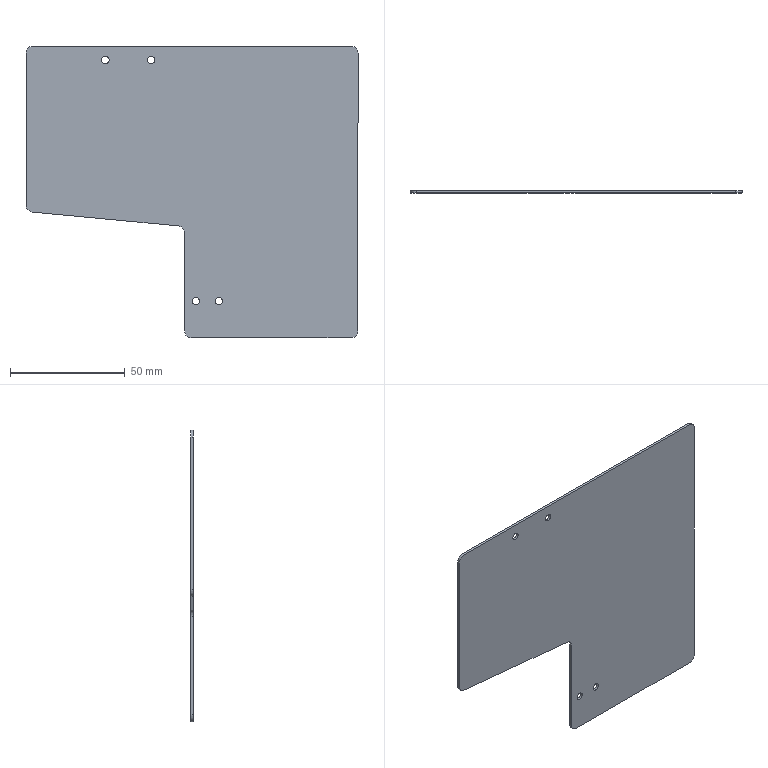Part | SolidWorks | features Extrusion 1, Fillet 1 | 1 solid | 22 faces | box 144.55 x 1 x 127 mm | volume 14747 mm3 | cylinder 14 | plane 8 | commonest cylinder face diameters 3.2 x8 6 x6
STEP:
#1=CARTESIAN_POINT('',(54.55,1.,-7.6));
#2=VERTEX_POINT('',#1);
#3=CARTESIAN_POINT('',(54.55,1.,-4.4));
#4=VERTEX_POINT('',#3);
#5=CARTESIAN_POINT('',(54.55,1.,-6.));
#6=DIRECTION('',(0.,1.,0.));
#7=DIRECTION('',(0.,0.,1.));
#8=AXIS2_PLACEMENT_3D('',#5,#6,#7);
#9=CIRCLE('',#8,1.6);
#10=EDGE_CURVE('',#2,#4,#9,.T.);
#11=ORIENTED_EDGE('',*,*,#10,.T.);
#12=CARTESIAN_POINT('',(54.55,0.,-4.4));
#13=VERTEX_POINT('',#12);
#14=CARTESIAN_POINT('',(54.55,1.,-4.4));
#15=DIRECTION('',(0.,-1.,0.));
#16=VECTOR('',#15,1000.);
#17=LINE('',#14,#16);
#18=EDGE_CURVE('',#4,#13,#17,.T.);
#19=ORIENTED_EDGE('',*,*,#18,.T.);
#20=CARTESIAN_POINT('',(54.55,0.,-7.6));
#21=VERTEX_POINT('',#20);
#22=CARTESIAN_POINT('',(54.55,0.,-6.));
#23=DIRECTION('',(0.,1.,0.));
#24=DIRECTION('',(0.,0.,1.));
#25=AXIS2_PLACEMENT_3D('',#22,#23,#24);
#26=CIRCLE('',#25,1.6);
#27=EDGE_CURVE('',#21,#13,#26,.T.);
#28=ORIENTED_EDGE('',*,*,#27,.F.);
#29=CARTESIAN_POINT('',(54.55,1.,-7.6));
#30=DIRECTION('',(0.,-1.,0.));
#31=VECTOR('',#30,1000.);
#32=LINE('',#29,#31);
#33=EDGE_CURVE('',#2,#21,#32,.T.);
#34=ORIENTED_EDGE('',*,*,#33,.F.);
#35=EDGE_LOOP('',(#11,#19,#28,#34));
#36=FACE_OUTER_BOUND('',#35,.T.);
#37=CARTESIAN_POINT('',(54.55,1.,-6.));
#38=DIRECTION('',(0.,-1.,0.));
#39=DIRECTION('',(0.,0.,-1.));
#40=AXIS2_PLACEMENT_3D('',#37,#38,#39);
#41=CYLINDRICAL_SURFACE('',#40,1.6);
#42=ADVANCED_FACE('',(#36),#41,.F.);
#43=CARTESIAN_POINT('',(34.55,1.,-7.6));
#44=VERTEX_POINT('',#43);
#45=CARTESIAN_POINT('',(34.55,1.,-4.4));
#46=VERTEX_POINT('',#45);
#47=CARTESIAN_POINT('',(34.55,1.,-6.));
#48=DIRECTION('',(0.,1.,0.));
#49=DIRECTION('',(0.,0.,1.));
#50=AXIS2_PLACEMENT_3D('',#47,#48,#49);
#51=CIRCLE('',#50,1.6);
#52=EDGE_CURVE('',#44,#46,#51,.T.);
#53=ORIENTED_EDGE('',*,*,#52,.T.);
#54=CARTESIAN_POINT('',(34.55,0.,-4.4));
#55=VERTEX_POINT('',#54);
#56=CARTESIAN_POINT('',(34.55,1.,-4.4));
#57=DIRECTION('',(0.,-1.,0.));
#58=VECTOR('',#57,1000.);
#59=LINE('',#56,#58);
#60=EDGE_CURVE('',#46,#55,#59,.T.);
#61=ORIENTED_EDGE('',*,*,#60,.T.);
#62=CARTESIAN_POINT('',(34.55,0.,-7.6));
#63=VERTEX_POINT('',#62);
#64=CARTESIAN_POINT('',(34.55,0.,-6.));
#65=DIRECTION('',(0.,1.,0.));
#66=DIRECTION('',(0.,0.,1.));
#67=AXIS2_PLACEMENT_3D('',#64,#65,#66);
#68=CIRCLE('',#67,1.6);
#69=EDGE_CURVE('',#63,#55,#68,.T.);
#70=ORIENTED_EDGE('',*,*,#69,.F.);
#71=CARTESIAN_POINT('',(34.55,1.,-7.6));
#72=DIRECTION('',(0.,-1.,0.));
#73=VECTOR('',#72,1000.);
#74=LINE('',#71,#73);
#75=EDGE_CURVE('',#44,#63,#74,.T.);
#76=ORIENTED_EDGE('',*,*,#75,.F.);
#77=EDGE_LOOP('',(#53,#61,#70,#76));
#78=FACE_OUTER_BOUND('',#77,.T.);
#79=CARTESIAN_POINT('',(34.55,1.,-6.));
#80=DIRECTION('',(0.,-1.,0.));
#81=DIRECTION('',(0.,0.,-1.));
#82=AXIS2_PLACEMENT_3D('',#79,#80,#81);
#83=CYLINDRICAL_SURFACE('',#82,1.6);
#84=ADVANCED_FACE('',(#78),#83,.F.);
#85=CARTESIAN_POINT('',(84.,1.,-112.6));
#86=VERTEX_POINT('',#85);
#87=CARTESIAN_POINT('',(84.,1.,-109.4));
#88=VERTEX_POINT('',#87);
#89=CARTESIAN_POINT('',(84.,1.,-111.));
#90=DIRECTION('',(0.,1.,0.));
#91=DIRECTION('',(0.,0.,1.));
#92=AXIS2_PLACEMENT_3D('',#89,#90,#91);
#93=CIRCLE('',#92,1.6);
#94=EDGE_CURVE('',#86,#88,#93,.T.);
#95=ORIENTED_EDGE('',*,*,#94,.T.);
#96=CARTESIAN_POINT('',(84.,0.,-109.4));
#97=VERTEX_POINT('',#96);
#98=CARTESIAN_POINT('',(84.,1.,-109.4));
#99=DIRECTION('',(0.,-1.,0.));
#100=VECTOR('',#99,1000.);
#101=LINE('',#98,#100);
#102=EDGE_CURVE('',#88,#97,#101,.T.);
#103=ORIENTED_EDGE('',*,*,#102,.T.);
#104=CARTESIAN_POINT('',(84.,0.,-112.6));
#105=VERTEX_POINT('',#104);
#106=CARTESIAN_POINT('',(84.,0.,-111.));
#107=DIRECTION('',(0.,1.,0.));
#108=DIRECTION('',(0.,0.,1.));
#109=AXIS2_PLACEMENT_3D('',#106,#107,#108);
#110=CIRCLE('',#109,1.6);
#111=EDGE_CURVE('',#105,#97,#110,.T.);
#112=ORIENTED_EDGE('',*,*,#111,.F.);
#113=CARTESIAN_POINT('',(84.,1.,-112.6));
#114=DIRECTION('',(0.,-1.,0.));
#115=VECTOR('',#114,1000.);
#116=LINE('',#113,#115);
#117=EDGE_CURVE('',#86,#105,#116,.T.);
#118=ORIENTED_EDGE('',*,*,#117,.F.);
#119=EDGE_LOOP('',(#95,#103,#112,#118));
#120=FACE_OUTER_BOUND('',#119,.T.);
#121=CARTESIAN_POINT('',(84.,1.,-111.));
#122=DIRECTION('',(0.,-1.,0.));
#123=DIRECTION('',(0.,0.,-1.));
#124=AXIS2_PLACEMENT_3D('',#121,#122,#123);
#125=CYLINDRICAL_SURFACE('',#124,1.6);
#126=ADVANCED_FACE('',(#120),#125,.F.);
#127=CARTESIAN_POINT('',(74.,1.,-112.6));
#128=VERTEX_POINT('',#127);
#129=CARTESIAN_POINT('',(74.,1.,-109.4));
#130=VERTEX_POINT('',#129);
#131=CARTESIAN_POINT('',(74.,1.,-111.));
#132=DIRECTION('',(0.,1.,0.));
#133=DIRECTION('',(0.,0.,1.));
#134=AXIS2_PLACEMENT_3D('',#131,#132,#133);
#135=CIRCLE('',#134,1.6);
#136=EDGE_CURVE('',#128,#130,#135,.T.);
#137=ORIENTED_EDGE('',*,*,#136,.T.);
#138=CARTESIAN_POINT('',(74.,0.,-109.4));
#139=VERTEX_POINT('',#138);
#140=CARTESIAN_POINT('',(74.,1.,-109.4));
#141=DIRECTION('',(0.,-1.,0.));
#142=VECTOR('',#141,1000.);
#143=LINE('',#140,#142);
#144=EDGE_CURVE('',#130,#139,#143,.T.);
#145=ORIENTED_EDGE('',*,*,#144,.T.);
#146=CARTESIAN_POINT('',(74.,0.,-112.6));
#147=VERTEX_POINT('',#146);
#148=CARTESIAN_POINT('',(74.,0.,-111.));
#149=DIRECTION('',(0.,1.,0.));
#150=DIRECTION('',(0.,0.,1.));
#151=AXIS2_PLACEMENT_3D('',#148,#149,#150);
#152=CIRCLE('',#151,1.6);
#153=EDGE_CURVE('',#147,#139,#152,.T.);
#154=ORIENTED_EDGE('',*,*,#153,.F.);
#155=CARTESIAN_POINT('',(74.,1.,-112.6));
#156=DIRECTION('',(0.,-1.,0.));
#157=VECTOR('',#156,1000.);
#158=LINE('',#155,#157);
#159=EDGE_CURVE('',#128,#147,#158,.T.);
#160=ORIENTED_EDGE('',*,*,#159,.F.);
#161=EDGE_LOOP('',(#137,#145,#154,#160));
#162=FACE_OUTER_BOUND('',#161,.T.);
#163=CARTESIAN_POINT('',(74.,1.,-111.));
#164=DIRECTION('',(0.,-1.,0.));
#165=DIRECTION('',(0.,0.,-1.));
#166=AXIS2_PLACEMENT_3D('',#163,#164,#165);
#167=CYLINDRICAL_SURFACE('',#166,1.6);
#168=ADVANCED_FACE('',(#162),#167,.F.);
#169=CARTESIAN_POINT('',(0.,1.,-69.269));
#170=VERTEX_POINT('',#169);
#171=CARTESIAN_POINT('',(0.,1.,-3.));
#172=VERTEX_POINT('',#171);
#173=CARTESIAN_POINT('',(0.,1.,0.));
#174=DIRECTION('',(0.,0.,1.));
#175=VECTOR('',#174,1000.);
#176=LINE('',#173,#175);
#177=EDGE_CURVE('',#170,#172,#176,.T.);
#178=ORIENTED_EDGE('',*,*,#177,.T.);
#179=CARTESIAN_POINT('',(3.,1.,0.));
#180=VERTEX_POINT('',#179);
#181=CARTESIAN_POINT('',(3.,1.,-3.));
#182=DIRECTION('',(0.,1.,0.));
#183=DIRECTION('',(0.,0.,-1.));
#184=AXIS2_PLACEMENT_3D('',#181,#182,#183);
#185=CIRCLE('',#184,3.);
#186=EDGE_CURVE('',#172,#180,#185,.T.);
#187=ORIENTED_EDGE('',*,*,#186,.T.);
#188=CARTESIAN_POINT('',(141.55,1.,0.));
#189=VERTEX_POINT('',#188);
#190=CARTESIAN_POINT('',(144.55,1.,0.));
#191=DIRECTION('',(1.,0.,0.));
#192=VECTOR('',#191,1000.);
#193=LINE('',#190,#192);
#194=EDGE_CURVE('',#180,#189,#193,.T.);
#195=ORIENTED_EDGE('',*,*,#194,.T.);
#196=CARTESIAN_POINT('',(144.55,1.,-3.));
#197=VERTEX_POINT('',#196);
#198=CARTESIAN_POINT('',(141.55,1.,-3.));
#199=DIRECTION('',(0.,1.,0.));
#200=DIRECTION('',(0.,0.,-1.));
#201=AXIS2_PLACEMENT_3D('',#198,#199,#200);
#202=CIRCLE('',#201,3.);
#203=EDGE_CURVE('',#189,#197,#202,.T.);
#204=ORIENTED_EDGE('',*,*,#203,.T.);
#205=CARTESIAN_POINT('',(144.55,1.,-124.));
#206=VERTEX_POINT('',#205);
#207=CARTESIAN_POINT('',(144.55,1.,-127.));
#208=DIRECTION('',(0.,0.,-1.));
#209=VECTOR('',#208,1000.);
#210=LINE('',#207,#209);
#211=EDGE_CURVE('',#197,#206,#210,.T.);
#212=ORIENTED_EDGE('',*,*,#211,.T.);
#213=CARTESIAN_POINT('',(141.55,1.,-127.));
#214=VERTEX_POINT('',#213);
#215=CARTESIAN_POINT('',(141.55,1.,-124.));
#216=DIRECTION('',(0.,1.,0.));
#217=DIRECTION('',(0.,0.,-1.));
#218=AXIS2_PLACEMENT_3D('',#215,#216,#217);
#219=CIRCLE('',#218,3.);
#220=EDGE_CURVE('',#206,#214,#219,.T.);
#221=ORIENTED_EDGE('',*,*,#220,.T.);
#222=CARTESIAN_POINT('',(72.,1.,-127.));
#223=VERTEX_POINT('',#222);
#224=CARTESIAN_POINT('',(69.,1.,-127.));
#225=DIRECTION('',(-1.,0.,0.));
#226=VECTOR('',#225,1000.);
#227=LINE('',#224,#226);
#228=EDGE_CURVE('',#214,#223,#227,.T.);
#229=ORIENTED_EDGE('',*,*,#228,.T.);
#230=CARTESIAN_POINT('',(69.,1.,-124.));
#231=VERTEX_POINT('',#230);
#232=CARTESIAN_POINT('',(72.,1.,-124.));
#233=DIRECTION('',(0.,1.,0.));
#234=DIRECTION('',(0.,0.,-1.));
#235=AXIS2_PLACEMENT_3D('',#232,#233,#234);
#236=CIRCLE('',#235,3.);
#237=EDGE_CURVE('',#223,#231,#236,.T.);
#238=ORIENTED_EDGE('',*,*,#237,.T.);
#239=CARTESIAN_POINT('',(69.,1.,-81.231));
#240=VERTEX_POINT('',#239);
#241=CARTESIAN_POINT('',(69.,1.,-78.5));
#242=DIRECTION('',(0.,0.,1.));
#243=VECTOR('',#242,1000.);
#244=LINE('',#241,#243);
#245=EDGE_CURVE('',#231,#240,#244,.T.);
#246=ORIENTED_EDGE('',*,*,#245,.T.);
#247=CARTESIAN_POINT('',(66.281,1.,-78.244));
#248=VERTEX_POINT('',#247);
#249=CARTESIAN_POINT('',(66.,1.,-81.231));
#250=DIRECTION('',(0.,-1.,0.));
#251=DIRECTION('',(0.,0.,-1.));
#252=AXIS2_PLACEMENT_3D('',#249,#250,#251);
#253=CIRCLE('',#252,3.);
#254=EDGE_CURVE('',#240,#248,#253,.T.);
#255=ORIENTED_EDGE('',*,*,#254,.T.);
#256=CARTESIAN_POINT('',(2.719,1.,-72.256));
#257=VERTEX_POINT('',#256);
#258=CARTESIAN_POINT('',(0.,1.,-72.));
#259=DIRECTION('',(-0.9956,0.,0.09379));
#260=VECTOR('',#259,1000.);
#261=LINE('',#258,#260);
#262=EDGE_CURVE('',#248,#257,#261,.T.);
#263=ORIENTED_EDGE('',*,*,#262,.T.);
#264=CARTESIAN_POINT('',(3.,1.,-69.269));
#265=DIRECTION('',(0.,1.,0.));
#266=DIRECTION('',(0.,0.,-1.));
#267=AXIS2_PLACEMENT_3D('',#264,#265,#266);
#268=CIRCLE('',#267,3.);
#269=EDGE_CURVE('',#257,#170,#268,.T.);
#270=ORIENTED_EDGE('',*,*,#269,.T.);
#271=EDGE_LOOP('',(#178,#187,#195,#204,#212,#221,#229,#238,#246,#255,#263,#270));
#272=FACE_OUTER_BOUND('',#271,.T.);
#273=ORIENTED_EDGE('',*,*,#136,.F.);
#274=CARTESIAN_POINT('',(74.,1.,-111.));
#275=DIRECTION('',(0.,1.,0.));
#276=DIRECTION('',(0.,0.,1.));
#277=AXIS2_PLACEMENT_3D('',#274,#275,#276);
#278=CIRCLE('',#277,1.6);
#279=EDGE_CURVE('',#130,#128,#278,.T.);
#280=ORIENTED_EDGE('',*,*,#279,.F.);
#281=EDGE_LOOP('',(#273,#280));
#282=FACE_BOUND('',#281,.T.);
#283=ORIENTED_EDGE('',*,*,#94,.F.);
#284=CARTESIAN_POINT('',(84.,1.,-111.));
#285=DIRECTION('',(0.,1.,0.));
#286=DIRECTION('',(0.,0.,1.));
#287=AXIS2_PLACEMENT_3D('',#284,#285,#286);
#288=CIRCLE('',#287,1.6);
#289=EDGE_CURVE('',#88,#86,#288,.T.);
#290=ORIENTED_EDGE('',*,*,#289,.F.);
#291=EDGE_LOOP('',(#283,#290));
#292=FACE_BOUND('',#291,.T.);
#293=ORIENTED_EDGE('',*,*,#52,.F.);
#294=CARTESIAN_POINT('',(34.55,1.,-6.));
#295=DIRECTION('',(0.,1.,0.));
#296=DIRECTION('',(0.,0.,1.));
#297=AXIS2_PLACEMENT_3D('',#294,#295,#296);
#298=CIRCLE('',#297,1.6);
#299=EDGE_CURVE('',#46,#44,#298,.T.);
#300=ORIENTED_EDGE('',*,*,#299,.F.);
#301=EDGE_LOOP('',(#293,#300));
#302=FACE_BOUND('',#301,.T.);
#303=ORIENTED_EDGE('',*,*,#10,.F.);
#304=CARTESIAN_POINT('',(54.55,1.,-6.));
#305=DIRECTION('',(0.,1.,0.));
#306=DIRECTION('',(0.,0.,1.));
#307=AXIS2_PLACEMENT_3D('',#304,#305,#306);
#308=CIRCLE('',#307,1.6);
#309=EDGE_CURVE('',#4,#2,#308,.T.);
#310=ORIENTED_EDGE('',*,*,#309,.F.);
#311=EDGE_LOOP('',(#303,#310));
#312=FACE_BOUND('',#311,.T.);
#313=CARTESIAN_POINT('',(0.,1.,0.));
#314=DIRECTION('',(0.,-1.,0.));
#315=DIRECTION('',(0.,0.,-1.));
#316=AXIS2_PLACEMENT_3D('',#313,#314,#315);
#317=PLANE('',#316);
#318=ADVANCED_FACE('',(#272,#282,#292,#302,#312),#317,.F.);
#319=ORIENTED_EDGE('',*,*,#69,.T.);
#320=CARTESIAN_POINT('',(34.55,0.,-6.));
#321=DIRECTION('',(0.,1.,0.));
#322=DIRECTION('',(0.,0.,1.));
#323=AXIS2_PLACEMENT_3D('',#320,#321,#322);
#324=CIRCLE('',#323,1.6);
#325=EDGE_CURVE('',#55,#63,#324,.T.);
#326=ORIENTED_EDGE('',*,*,#325,.T.);
#327=EDGE_LOOP('',(#319,#326));
#328=FACE_BOUND('',#327,.T.);
#329=ORIENTED_EDGE('',*,*,#153,.T.);
#330=CARTESIAN_POINT('',(74.,0.,-111.));
#331=DIRECTION('',(0.,1.,0.));
#332=DIRECTION('',(0.,0.,1.));
#333=AXIS2_PLACEMENT_3D('',#330,#331,#332);
#334=CIRCLE('',#333,1.6);
#335=EDGE_CURVE('',#139,#147,#334,.T.);
#336=ORIENTED_EDGE('',*,*,#335,.T.);
#337=EDGE_LOOP('',(#329,#336));
#338=FACE_BOUND('',#337,.T.);
#339=CARTESIAN_POINT('',(3.,0.,0.));
#340=VERTEX_POINT('',#339);
#341=CARTESIAN_POINT('',(141.55,0.,0.));
#342=VERTEX_POINT('',#341);
#343=CARTESIAN_POINT('',(144.55,0.,0.));
#344=DIRECTION('',(1.,0.,0.));
#345=VECTOR('',#344,1000.);
#346=LINE('',#343,#345);
#347=EDGE_CURVE('',#340,#342,#346,.T.);
#348=ORIENTED_EDGE('',*,*,#347,.F.);
#349=CARTESIAN_POINT('',(0.,0.,-3.));
#350=VERTEX_POINT('',#349);
#351=CARTESIAN_POINT('',(3.,0.,-3.));
#352=DIRECTION('',(0.,-1.,0.));
#353=DIRECTION('',(0.,0.,-1.));
#354=AXIS2_PLACEMENT_3D('',#351,#352,#353);
#355=CIRCLE('',#354,3.);
#356=EDGE_CURVE('',#340,#350,#355,.T.);
#357=ORIENTED_EDGE('',*,*,#356,.T.);
#358=CARTESIAN_POINT('',(0.,0.,-69.269));
#359=VERTEX_POINT('',#358);
#360=CARTESIAN_POINT('',(0.,0.,0.));
#361=DIRECTION('',(0.,0.,1.));
#362=VECTOR('',#361,1000.);
#363=LINE('',#360,#362);
#364=EDGE_CURVE('',#359,#350,#363,.T.);
#365=ORIENTED_EDGE('',*,*,#364,.F.);
#366=CARTESIAN_POINT('',(2.719,0.,-72.256));
#367=VERTEX_POINT('',#366);
#368=CARTESIAN_POINT('',(3.,0.,-69.269));
#369=DIRECTION('',(0.,-1.,0.));
#370=DIRECTION('',(0.,0.,-1.));
#371=AXIS2_PLACEMENT_3D('',#368,#369,#370);
#372=CIRCLE('',#371,3.);
#373=EDGE_CURVE('',#359,#367,#372,.T.);
#374=ORIENTED_EDGE('',*,*,#373,.T.);
#375=CARTESIAN_POINT('',(66.281,0.,-78.244));
#376=VERTEX_POINT('',#375);
#377=CARTESIAN_POINT('',(0.,0.,-72.));
#378=DIRECTION('',(-0.9956,0.,0.09379));
#379=VECTOR('',#378,1000.);
#380=LINE('',#377,#379);
#381=EDGE_CURVE('',#376,#367,#380,.T.);
#382=ORIENTED_EDGE('',*,*,#381,.F.);
#383=CARTESIAN_POINT('',(69.,0.,-81.231));
#384=VERTEX_POINT('',#383);
#385=CARTESIAN_POINT('',(66.,0.,-81.231));
#386=DIRECTION('',(0.,1.,0.));
#387=DIRECTION('',(0.,0.,-1.));
#388=AXIS2_PLACEMENT_3D('',#385,#386,#387);
#389=CIRCLE('',#388,3.);
#390=EDGE_CURVE('',#376,#384,#389,.T.);
#391=ORIENTED_EDGE('',*,*,#390,.T.);
#392=CARTESIAN_POINT('',(69.,0.,-124.));
#393=VERTEX_POINT('',#392);
#394=CARTESIAN_POINT('',(69.,0.,-78.5));
#395=DIRECTION('',(0.,0.,1.));
#396=VECTOR('',#395,1000.);
#397=LINE('',#394,#396);
#398=EDGE_CURVE('',#393,#384,#397,.T.);
#399=ORIENTED_EDGE('',*,*,#398,.F.);
#400=CARTESIAN_POINT('',(72.,0.,-127.));
#401=VERTEX_POINT('',#400);
#402=CARTESIAN_POINT('',(72.,0.,-124.));
#403=DIRECTION('',(0.,-1.,0.));
#404=DIRECTION('',(0.,0.,-1.));
#405=AXIS2_PLACEMENT_3D('',#402,#403,#404);
#406=CIRCLE('',#405,3.);
#407=EDGE_CURVE('',#393,#401,#406,.T.);
#408=ORIENTED_EDGE('',*,*,#407,.T.);
#409=CARTESIAN_POINT('',(141.55,0.,-127.));
#410=VERTEX_POINT('',#409);
#411=CARTESIAN_POINT('',(69.,0.,-127.));
#412=DIRECTION('',(-1.,0.,0.));
#413=VECTOR('',#412,1000.);
#414=LINE('',#411,#413);
#415=EDGE_CURVE('',#410,#401,#414,.T.);
#416=ORIENTED_EDGE('',*,*,#415,.F.);
#417=CARTESIAN_POINT('',(144.55,0.,-124.));
#418=VERTEX_POINT('',#417);
#419=CARTESIAN_POINT('',(141.55,0.,-124.));
#420=DIRECTION('',(0.,-1.,0.));
#421=DIRECTION('',(0.,0.,-1.));
#422=AXIS2_PLACEMENT_3D('',#419,#420,#421);
#423=CIRCLE('',#422,3.);
#424=EDGE_CURVE('',#410,#418,#423,.T.);
#425=ORIENTED_EDGE('',*,*,#424,.T.);
#426=CARTESIAN_POINT('',(144.55,0.,-3.));
#427=VERTEX_POINT('',#426);
#428=CARTESIAN_POINT('',(144.55,0.,-127.));
#429=DIRECTION('',(0.,0.,-1.));
#430=VECTOR('',#429,1000.);
#431=LINE('',#428,#430);
#432=EDGE_CURVE('',#427,#418,#431,.T.);
#433=ORIENTED_EDGE('',*,*,#432,.F.);
#434=CARTESIAN_POINT('',(141.55,0.,-3.));
#435=DIRECTION('',(0.,-1.,0.));
#436=DIRECTION('',(0.,0.,-1.));
#437=AXIS2_PLACEMENT_3D('',#434,#435,#436);
#438=CIRCLE('',#437,3.);
#439=EDGE_CURVE('',#427,#342,#438,.T.);
#440=ORIENTED_EDGE('',*,*,#439,.T.);
#441=EDGE_LOOP('',(#348,#357,#365,#374,#382,#391,#399,#408,#416,#425,#433,#440));
#442=FACE_OUTER_BOUND('',#441,.T.);
#443=ORIENTED_EDGE('',*,*,#111,.T.);
#444=CARTESIAN_POINT('',(84.,0.,-111.));
#445=DIRECTION('',(0.,1.,0.));
#446=DIRECTION('',(0.,0.,1.));
#447=AXIS2_PLACEMENT_3D('',#444,#445,#446);
#448=CIRCLE('',#447,1.6);
#449=EDGE_CURVE('',#97,#105,#448,.T.);
#450=ORIENTED_EDGE('',*,*,#449,.T.);
#451=EDGE_LOOP('',(#443,#450));
#452=FACE_BOUND('',#451,.T.);
#453=ORIENTED_EDGE('',*,*,#27,.T.);
#454=CARTESIAN_POINT('',(54.55,0.,-6.));
#455=DIRECTION('',(0.,1.,0.));
#456=DIRECTION('',(0.,0.,1.));
#457=AXIS2_PLACEMENT_3D('',#454,#455,#456);
#458=CIRCLE('',#457,1.6);
#459=EDGE_CURVE('',#13,#21,#458,.T.);
#460=ORIENTED_EDGE('',*,*,#459,.T.);
#461=EDGE_LOOP('',(#453,#460));
#462=FACE_BOUND('',#461,.T.);
#463=CARTESIAN_POINT('',(0.,0.,0.));
#464=DIRECTION('',(0.,-1.,0.));
#465=DIRECTION('',(0.,0.,-1.));
#466=AXIS2_PLACEMENT_3D('',#463,#464,#465);
#467=PLANE('',#466);
#468=ADVANCED_FACE('',(#328,#338,#442,#452,#462),#467,.T.);
#469=ORIENTED_EDGE('',*,*,#194,.F.);
#470=CARTESIAN_POINT('',(3.,1.,0.));
#471=DIRECTION('',(0.,-1.,0.));
#472=VECTOR('',#471,1000.);
#473=LINE('',#470,#472);
#474=EDGE_CURVE('',#180,#340,#473,.T.);
#475=ORIENTED_EDGE('',*,*,#474,.T.);
#476=ORIENTED_EDGE('',*,*,#347,.T.);
#477=CARTESIAN_POINT('',(141.55,1.,0.));
#478=DIRECTION('',(0.,1.,0.));
#479=VECTOR('',#478,1000.);
#480=LINE('',#477,#479);
#481=EDGE_CURVE('',#342,#189,#480,.T.);
#482=ORIENTED_EDGE('',*,*,#481,.T.);
#483=EDGE_LOOP('',(#469,#475,#476,#482));
#484=FACE_OUTER_BOUND('',#483,.T.);
#485=CARTESIAN_POINT('',(144.55,1.,0.));
#486=DIRECTION('',(0.,0.,-1.));
#487=DIRECTION('',(-1.,0.,0.));
#488=AXIS2_PLACEMENT_3D('',#485,#486,#487);
#489=PLANE('',#488);
#490=ADVANCED_FACE('',(#484),#489,.F.);
#491=ORIENTED_EDGE('',*,*,#432,.T.);
#492=CARTESIAN_POINT('',(144.55,1.,-124.));
#493=DIRECTION('',(0.,1.,0.));
#494=VECTOR('',#493,1000.);
#495=LINE('',#492,#494);
#496=EDGE_CURVE('',#418,#206,#495,.T.);
#497=ORIENTED_EDGE('',*,*,#496,.T.);
#498=ORIENTED_EDGE('',*,*,#211,.F.);
#499=CARTESIAN_POINT('',(144.55,1.,-3.));
#500=DIRECTION('',(0.,-1.,0.));
#501=VECTOR('',#500,1000.);
#502=LINE('',#499,#501);
#503=EDGE_CURVE('',#197,#427,#502,.T.);
#504=ORIENTED_EDGE('',*,*,#503,.T.);
#505=EDGE_LOOP('',(#491,#497,#498,#504));
#506=FACE_OUTER_BOUND('',#505,.T.);
#507=CARTESIAN_POINT('',(144.55,1.,-127.));
#508=DIRECTION('',(-1.,0.,0.));
#509=DIRECTION('',(0.,0.,1.));
#510=AXIS2_PLACEMENT_3D('',#507,#508,#509);
#511=PLANE('',#510);
#512=ADVANCED_FACE('',(#506),#511,.F.);
#513=ORIENTED_EDGE('',*,*,#415,.T.);
#514=CARTESIAN_POINT('',(72.,1.,-127.));
#515=DIRECTION('',(0.,1.,0.));
#516=VECTOR('',#515,1000.);
#517=LINE('',#514,#516);
#518=EDGE_CURVE('',#401,#223,#517,.T.);
#519=ORIENTED_EDGE('',*,*,#518,.T.);
#520=ORIENTED_EDGE('',*,*,#228,.F.);
#521=CARTESIAN_POINT('',(141.55,1.,-127.));
#522=DIRECTION('',(0.,-1.,0.));
#523=VECTOR('',#522,1000.);
#524=LINE('',#521,#523);
#525=EDGE_CURVE('',#214,#410,#524,.T.);
#526=ORIENTED_EDGE('',*,*,#525,.T.);
#527=EDGE_LOOP('',(#513,#519,#520,#526));
#528=FACE_OUTER_BOUND('',#527,.T.);
#529=CARTESIAN_POINT('',(69.,1.,-127.));
#530=DIRECTION('',(0.,0.,1.));
#531=DIRECTION('',(1.,0.,0.));
#532=AXIS2_PLACEMENT_3D('',#529,#530,#531);
#533=PLANE('',#532);
#534=ADVANCED_FACE('',(#528),#533,.F.);
#535=ORIENTED_EDGE('',*,*,#398,.T.);
#536=CARTESIAN_POINT('',(69.,1.,-81.231));
#537=DIRECTION('',(0.,1.,0.));
#538=VECTOR('',#537,1000.);
#539=LINE('',#536,#538);
#540=EDGE_CURVE('',#384,#240,#539,.T.);
#541=ORIENTED_EDGE('',*,*,#540,.T.);
#542=ORIENTED_EDGE('',*,*,#245,.F.);
#543=CARTESIAN_POINT('',(69.,1.,-124.));
#544=DIRECTION('',(0.,-1.,0.));
#545=VECTOR('',#544,1000.);
#546=LINE('',#543,#545);
#547=EDGE_CURVE('',#231,#393,#546,.T.);
#548=ORIENTED_EDGE('',*,*,#547,.T.);
#549=EDGE_LOOP('',(#535,#541,#542,#548));
#550=FACE_OUTER_BOUND('',#549,.T.);
#551=CARTESIAN_POINT('',(69.,1.,-78.5));
#552=DIRECTION('',(1.,0.,0.));
#553=DIRECTION('',(0.,0.,-1.));
#554=AXIS2_PLACEMENT_3D('',#551,#552,#553);
#555=PLANE('',#554);
#556=ADVANCED_FACE('',(#550),#555,.F.);
#557=ORIENTED_EDGE('',*,*,#381,.T.);
#558=CARTESIAN_POINT('',(2.719,1.,-72.256));
#559=DIRECTION('',(0.,1.,0.));
#560=VECTOR('',#559,1000.);
#561=LINE('',#558,#560);
#562=EDGE_CURVE('',#367,#257,#561,.T.);
#563=ORIENTED_EDGE('',*,*,#562,.T.);
#564=ORIENTED_EDGE('',*,*,#262,.F.);
#565=CARTESIAN_POINT('',(66.281,0.,-78.244));
#566=DIRECTION('',(0.,-1.,0.));
#567=VECTOR('',#566,1000.);
#568=LINE('',#565,#567);
#569=EDGE_CURVE('',#248,#376,#568,.T.);
#570=ORIENTED_EDGE('',*,*,#569,.T.);
#571=EDGE_LOOP('',(#557,#563,#564,#570));
#572=FACE_OUTER_BOUND('',#571,.T.);
#573=CARTESIAN_POINT('',(0.,1.,-72.));
#574=DIRECTION('',(0.09379,0.,0.9956));
#575=DIRECTION('',(0.9956,0.,-0.09379));
#576=AXIS2_PLACEMENT_3D('',#573,#574,#575);
#577=PLANE('',#576);
#578=ADVANCED_FACE('',(#572),#577,.F.);
#579=ORIENTED_EDGE('',*,*,#364,.T.);
#580=CARTESIAN_POINT('',(0.,1.,-3.));
#581=DIRECTION('',(0.,1.,0.));
#582=VECTOR('',#581,1000.);
#583=LINE('',#580,#582);
#584=EDGE_CURVE('',#350,#172,#583,.T.);
#585=ORIENTED_EDGE('',*,*,#584,.T.);
#586=ORIENTED_EDGE('',*,*,#177,.F.);
#587=CARTESIAN_POINT('',(0.,1.,-69.269));
#588=DIRECTION('',(0.,-1.,0.));
#589=VECTOR('',#588,1000.);
#590=LINE('',#587,#589);
#591=EDGE_CURVE('',#170,#359,#590,.T.);
#592=ORIENTED_EDGE('',*,*,#591,.T.);
#593=EDGE_LOOP('',(#579,#585,#586,#592));
#594=FACE_OUTER_BOUND('',#593,.T.);
#595=CARTESIAN_POINT('',(0.,1.,0.));
#596=DIRECTION('',(1.,0.,0.));
#597=DIRECTION('',(0.,0.,-1.));
#598=AXIS2_PLACEMENT_3D('',#595,#596,#597);
#599=PLANE('',#598);
#600=ADVANCED_FACE('',(#594),#599,.F.);
#601=ORIENTED_EDGE('',*,*,#144,.F.);
#602=ORIENTED_EDGE('',*,*,#279,.T.);
#603=ORIENTED_EDGE('',*,*,#159,.T.);
#604=ORIENTED_EDGE('',*,*,#335,.F.);
#605=EDGE_LOOP('',(#601,#602,#603,#604));
#606=FACE_OUTER_BOUND('',#605,.T.);
#607=CARTESIAN_POINT('',(74.,1.,-111.));
#608=DIRECTION('',(0.,-1.,0.));
#609=DIRECTION('',(0.,0.,-1.));
#610=AXIS2_PLACEMENT_3D('',#607,#608,#609);
#611=CYLINDRICAL_SURFACE('',#610,1.6);
#612=ADVANCED_FACE('',(#606),#611,.F.);
#613=ORIENTED_EDGE('',*,*,#102,.F.);
#614=ORIENTED_EDGE('',*,*,#289,.T.);
#615=ORIENTED_EDGE('',*,*,#117,.T.);
#616=ORIENTED_EDGE('',*,*,#449,.F.);
#617=EDGE_LOOP('',(#613,#614,#615,#616));
#618=FACE_OUTER_BOUND('',#617,.T.);
#619=CARTESIAN_POINT('',(84.,1.,-111.));
#620=DIRECTION('',(0.,-1.,0.));
#621=DIRECTION('',(0.,0.,-1.));
#622=AXIS2_PLACEMENT_3D('',#619,#620,#621);
#623=CYLINDRICAL_SURFACE('',#622,1.6);
#624=ADVANCED_FACE('',(#618),#623,.F.);
#625=ORIENTED_EDGE('',*,*,#60,.F.);
#626=ORIENTED_EDGE('',*,*,#299,.T.);
#627=ORIENTED_EDGE('',*,*,#75,.T.);
#628=ORIENTED_EDGE('',*,*,#325,.F.);
#629=EDGE_LOOP('',(#625,#626,#627,#628));
#630=FACE_OUTER_BOUND('',#629,.T.);
#631=CARTESIAN_POINT('',(34.55,1.,-6.));
#632=DIRECTION('',(0.,-1.,0.));
#633=DIRECTION('',(0.,0.,-1.));
#634=AXIS2_PLACEMENT_3D('',#631,#632,#633);
#635=CYLINDRICAL_SURFACE('',#634,1.6);
#636=ADVANCED_FACE('',(#630),#635,.F.);
#637=ORIENTED_EDGE('',*,*,#18,.F.);
#638=ORIENTED_EDGE('',*,*,#309,.T.);
#639=ORIENTED_EDGE('',*,*,#33,.T.);
#640=ORIENTED_EDGE('',*,*,#459,.F.);
#641=EDGE_LOOP('',(#637,#638,#639,#640));
#642=FACE_OUTER_BOUND('',#641,.T.);
#643=CARTESIAN_POINT('',(54.55,1.,-6.));
#644=DIRECTION('',(0.,-1.,0.));
#645=DIRECTION('',(0.,0.,-1.));
#646=AXIS2_PLACEMENT_3D('',#643,#644,#645);
#647=CYLINDRICAL_SURFACE('',#646,1.6);
#648=ADVANCED_FACE('',(#642),#647,.F.);
#649=ORIENTED_EDGE('',*,*,#186,.F.);
#650=ORIENTED_EDGE('',*,*,#584,.F.);
#651=ORIENTED_EDGE('',*,*,#356,.F.);
#652=ORIENTED_EDGE('',*,*,#474,.F.);
#653=EDGE_LOOP('',(#649,#650,#651,#652));
#654=FACE_OUTER_BOUND('',#653,.T.);
#655=CARTESIAN_POINT('',(3.,1.,-3.));
#656=DIRECTION('',(0.,-1.,0.));
#657=DIRECTION('',(0.,0.,-1.));
#658=AXIS2_PLACEMENT_3D('',#655,#656,#657);
#659=CYLINDRICAL_SURFACE('',#658,3.);
#660=ADVANCED_FACE('',(#654),#659,.T.);
#661=ORIENTED_EDGE('',*,*,#269,.F.);
#662=ORIENTED_EDGE('',*,*,#562,.F.);
#663=ORIENTED_EDGE('',*,*,#373,.F.);
#664=ORIENTED_EDGE('',*,*,#591,.F.);
#665=EDGE_LOOP('',(#661,#662,#663,#664));
#666=FACE_OUTER_BOUND('',#665,.T.);
#667=CARTESIAN_POINT('',(3.,1.,-69.269));
#668=DIRECTION('',(0.,-1.,0.));
#669=DIRECTION('',(0.,0.,-1.));
#670=AXIS2_PLACEMENT_3D('',#667,#668,#669);
#671=CYLINDRICAL_SURFACE('',#670,3.);
#672=ADVANCED_FACE('',(#666),#671,.T.);
#673=ORIENTED_EDGE('',*,*,#254,.F.);
#674=ORIENTED_EDGE('',*,*,#540,.F.);
#675=ORIENTED_EDGE('',*,*,#390,.F.);
#676=ORIENTED_EDGE('',*,*,#569,.F.);
#677=EDGE_LOOP('',(#673,#674,#675,#676));
#678=FACE_OUTER_BOUND('',#677,.T.);
#679=CARTESIAN_POINT('',(66.,1.,-81.231));
#680=DIRECTION('',(0.,1.,0.));
#681=DIRECTION('',(0.,0.,1.));
#682=AXIS2_PLACEMENT_3D('',#679,#680,#681);
#683=CYLINDRICAL_SURFACE('',#682,3.);
#684=ADVANCED_FACE('',(#678),#683,.F.);
#685=ORIENTED_EDGE('',*,*,#237,.F.);
#686=ORIENTED_EDGE('',*,*,#518,.F.);
#687=ORIENTED_EDGE('',*,*,#407,.F.);
#688=ORIENTED_EDGE('',*,*,#547,.F.);
#689=EDGE_LOOP('',(#685,#686,#687,#688));
#690=FACE_OUTER_BOUND('',#689,.T.);
#691=CARTESIAN_POINT('',(72.,1.,-124.));
#692=DIRECTION('',(0.,-1.,0.));
#693=DIRECTION('',(0.,0.,-1.));
#694=AXIS2_PLACEMENT_3D('',#691,#692,#693);
#695=CYLINDRICAL_SURFACE('',#694,3.);
#696=ADVANCED_FACE('',(#690),#695,.T.);
#697=ORIENTED_EDGE('',*,*,#220,.F.);
#698=ORIENTED_EDGE('',*,*,#496,.F.);
#699=ORIENTED_EDGE('',*,*,#424,.F.);
#700=ORIENTED_EDGE('',*,*,#525,.F.);
#701=EDGE_LOOP('',(#697,#698,#699,#700));
#702=FACE_OUTER_BOUND('',#701,.T.);
#703=CARTESIAN_POINT('',(141.55,1.,-124.));
#704=DIRECTION('',(0.,-1.,0.));
#705=DIRECTION('',(0.,0.,-1.));
#706=AXIS2_PLACEMENT_3D('',#703,#704,#705);
#707=CYLINDRICAL_SURFACE('',#706,3.);
#708=ADVANCED_FACE('',(#702),#707,.T.);
#709=ORIENTED_EDGE('',*,*,#203,.F.);
#710=ORIENTED_EDGE('',*,*,#481,.F.);
#711=ORIENTED_EDGE('',*,*,#439,.F.);
#712=ORIENTED_EDGE('',*,*,#503,.F.);
#713=EDGE_LOOP('',(#709,#710,#711,#712));
#714=FACE_OUTER_BOUND('',#713,.T.);
#715=CARTESIAN_POINT('',(141.55,1.,-3.));
#716=DIRECTION('',(0.,-1.,0.));
#717=DIRECTION('',(0.,0.,-1.));
#718=AXIS2_PLACEMENT_3D('',#715,#716,#717);
#719=CYLINDRICAL_SURFACE('',#718,3.);
#720=ADVANCED_FACE('',(#714),#719,.T.);
#721=CLOSED_SHELL('',(#42,#84,#126,#168,#318,#468,#490,#512,#534,#556,#578,#600,#612,#624,#636,#648,#660,#672,#684,#696,#708,#720));
#722=MANIFOLD_SOLID_BREP('',#721);
#723=CARTESIAN_POINT('',(0.,0.,0.));
#724=DIRECTION('',(0.,0.,1.));
#725=DIRECTION('',(1.,0.,0.));
#726=AXIS2_PLACEMENT_3D('',#723,#724,#725);
#727=(LENGTH_UNIT()NAMED_UNIT(*)SI_UNIT(.MILLI.,.METRE.));
#728=UNCERTAINTY_MEASURE_WITH_UNIT(LENGTH_MEASURE(0.00001),#727,'','');
#729=(NAMED_UNIT(*)PLANE_ANGLE_UNIT()SI_UNIT($,.RADIAN.));
#730=(NAMED_UNIT(*)SI_UNIT($,.STERADIAN.)SOLID_ANGLE_UNIT());
#731=(GEOMETRIC_REPRESENTATION_CONTEXT(3)GLOBAL_UNCERTAINTY_ASSIGNED_CONTEXT((#728))GLOBAL_UNIT_ASSIGNED_CONTEXT((#727,#729,#730))REPRESENTATION_CONTEXT('',''));
#732=ADVANCED_BREP_SHAPE_REPRESENTATION('',(#722,#726),#731);